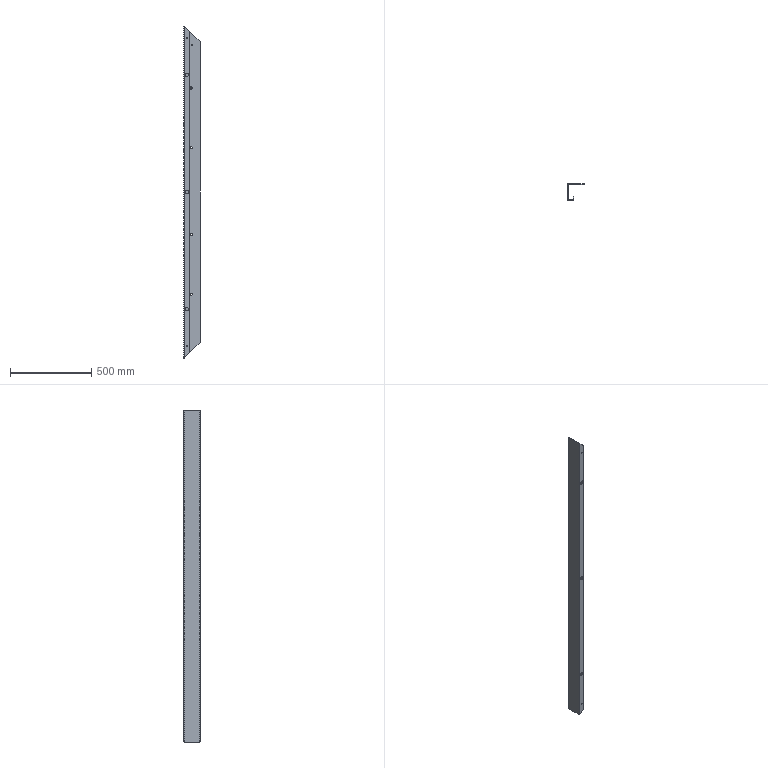Part | STEP file | HESS-408-70-15W-W-13-bottom frame 3 | 1 solid | 62 faces | box 100 x 100 x 2039 mm | volume 1445665 mm3 | cylinder 36 | plane 22 | spline 4 | commonest cylinder face diameters 15 x8 3.3 x6 6.8 x6 22 x6 5 x4 0.2 x3